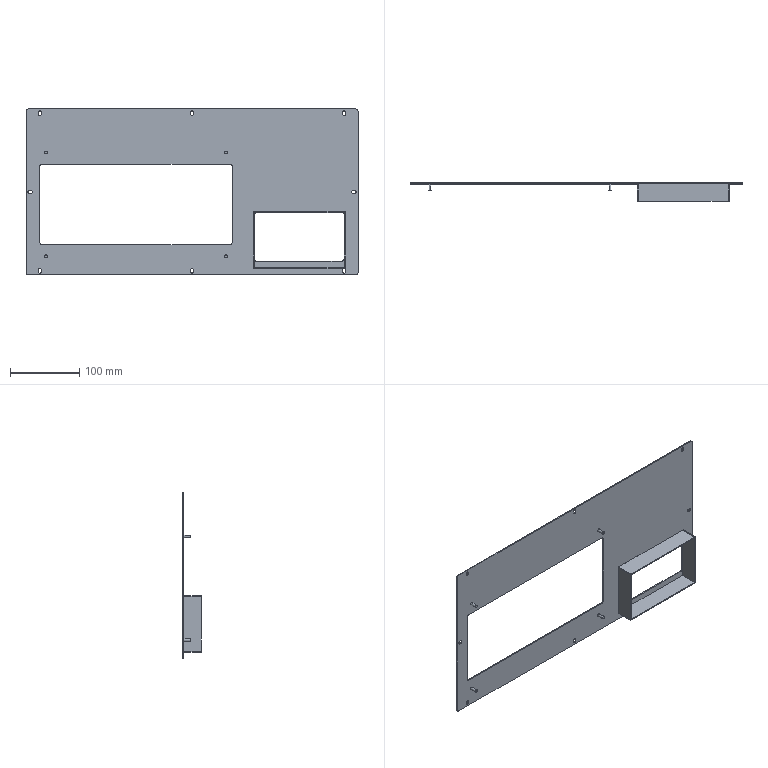Part | NX | features BREP 5 | 5 solids | 100 faces | box 480 x 26.5 x 240 mm | volume 126845 mm3 | plane 58 | cylinder 42 | commonest cylinder face diameters 4.6 x22 6 x12 4 x8